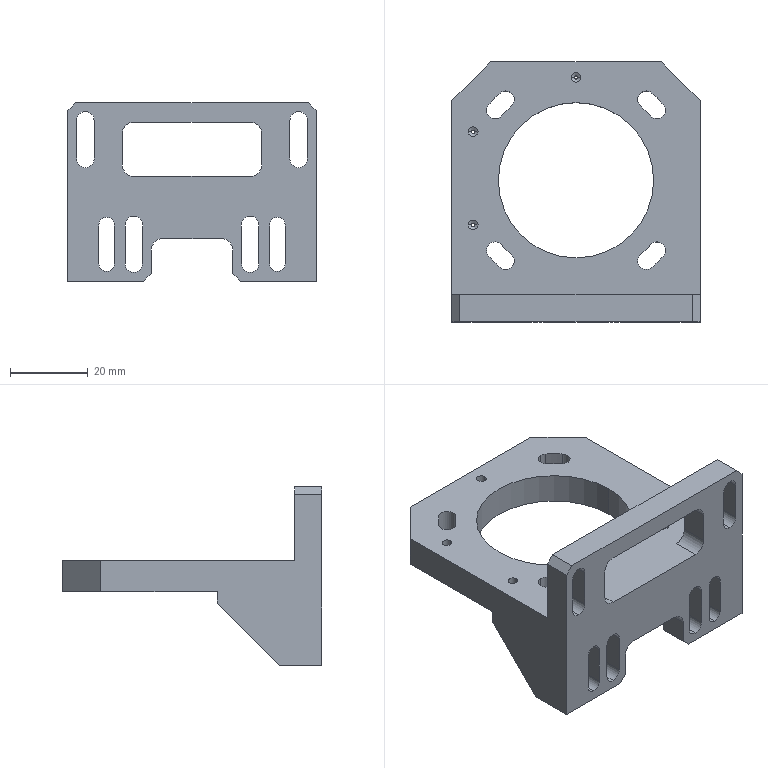NC program | NX | posted with a generic post | part box 64 x 67 x 46 mm
Lines 1 to 508 of 8734:
N10 G17 G21 G94 G90
(ZLEVEL_PROFILE_COPY_3 , TOOL : D10C)
N12 T10 M6
N14 G54
N16 G17 G0 G90 X12.9 Y-10.028 B0. C0. S2500 M3
N18 G43 Z30. H10
N20 Z1.5
N22 G94 G1 Y-9.141 Z1.454 F1000.
N24 X12.902 Y-9.1 Z1.451
N26 X-12.9 Z0.099
N28 Y-12.9 Z-0.1
N30 X12.902 F2500.
N32 X12.9 Y-12.855
N34 Y-9.141
N36 X12.902 Y-9.1
N38 X-12.9
N40 Y-12.9
N42 X-7.171 Z-0.2
N44 X12.902
N46 X12.9 Y-12.855
N48 Y-9.141
N50 X12.902 Y-9.1
N52 X-12.9
N54 Y-12.9
N56 X-7.171 Z-0.3
N58 X12.902
N60 X12.9 Y-12.855
N62 Y-9.141
N64 X12.902 Y-9.1
N66 X-12.9
N68 Y-12.9
N70 X-7.171 Z-0.4
N72 X12.902
N74 X12.9 Y-12.855
N76 Y-9.141
N78 X12.902 Y-9.1
N80 X-12.9
N82 Y-12.9
N84 X-7.171 Z-0.5
N86 X12.902
N88 X12.9 Y-12.855
N90 Y-9.141
N92 X12.902 Y-9.1
N94 X-12.9
N96 Y-12.9
N98 X-7.171 Z-0.6
N100 X12.902
N102 X12.9 Y-12.855
N104 Y-9.141
N106 X12.902 Y-9.1
N108 X-12.9
N110 Y-12.9
N112 X-7.171 Z-0.7
N114 X12.902
N116 X12.9 Y-12.855
N118 Y-9.141
N120 X12.902 Y-9.1
N122 X-12.9
N124 Y-12.9
N126 X-7.171 Z-0.8
N128 X12.902
N130 X12.9 Y-12.855
N132 Y-9.141
N134 X12.902 Y-9.1
N136 X-12.9
N138 Y-12.9
N140 X-7.171 Z-0.9
N142 X12.902
N144 X12.9 Y-12.855
N146 Y-9.141
N148 X12.902 Y-9.1
N150 X-12.9
N152 Y-12.9
N154 X-7.171 Z-1.
N156 X12.902
N158 X12.9 Y-12.855
N160 Y-9.141
N162 X12.902 Y-9.1
N164 X-12.9
N166 Y-12.9
N168 X-7.171 Z-1.1
N170 X12.902
N172 X12.9 Y-12.855
N174 Y-9.141
N176 X12.902 Y-9.1
N178 X-12.9
N180 Y-12.9
N182 X-7.171 Z-1.2
N184 X12.902
N186 X12.9 Y-12.855
N188 Y-9.141
N190 X12.902 Y-9.1
N192 X-12.9
N194 Y-12.9
N196 X-7.171 Z-1.3
N198 X12.902
N200 X12.9 Y-12.855
N202 Y-9.141
N204 X12.902 Y-9.1
N206 X-12.9
N208 Y-12.9
N210 X-7.171 Z-1.4
N212 X12.902
N214 X12.9 Y-12.855
N216 Y-9.141
N218 X12.902 Y-9.1
N220 X-12.9
N222 Y-12.9
N224 X-7.171 Z-1.5
N226 X12.902
N228 X12.9 Y-12.855
N230 Y-9.141
N232 X12.902 Y-9.1
N234 X-12.9
N236 Y-12.9
N238 X-7.171 Z-1.6
N240 X12.902
N242 X12.9 Y-12.855
N244 Y-9.141
N246 X12.902 Y-9.1
N248 X-12.9
N250 Y-12.9
N252 X-7.171 Z-1.7
N254 X12.902
N256 X12.9 Y-12.855
N258 Y-9.141
N260 X12.902 Y-9.1
N262 X-12.9
N264 Y-12.9
N266 X-7.171 Z-1.8
N268 X12.902
N270 X12.9 Y-12.855
N272 Y-9.141
N274 X12.902 Y-9.1
N276 X-12.9
N278 Y-12.9
N280 X-7.171 Z-1.9
N282 X12.902
N284 X12.9 Y-12.855
N286 Y-9.141
N288 X12.902 Y-9.1
N290 X-12.9
N292 Y-12.9
N294 X-7.171 Z-2.
N296 X12.902
N298 X12.9 Y-12.855
N300 Y-9.141
N302 X12.902 Y-9.1
N304 X-12.9
N306 Y-12.9
N308 X-7.171 Z-2.1
N310 X12.902
N312 X12.9 Y-12.855
N314 Y-9.141
N316 X12.902 Y-9.1
N318 X-12.9
N320 Y-12.9
N322 X-7.171 Z-2.2
N324 X12.902
N326 X12.9 Y-12.855
N328 Y-9.141
N330 X12.902 Y-9.1
N332 X-12.9
N334 Y-12.9
N336 X-7.171 Z-2.3
N338 X12.902
N340 X12.9 Y-12.855
N342 Y-9.141
N344 X12.902 Y-9.1
N346 X-12.9
N348 Y-12.9
N350 X-7.171 Z-2.4
N352 X12.902
N354 X12.9 Y-12.855
N356 Y-9.141
N358 X12.902 Y-9.1
N360 X-12.9
N362 Y-12.9
N364 X-7.171 Z-2.5
N366 X12.902
N368 X12.9 Y-12.855
N370 Y-9.141
N372 X12.902 Y-9.1
N374 X-12.9
N376 Y-12.9
N378 X-7.171 Z-2.6
N380 X12.902
N382 X12.9 Y-12.855
N384 Y-9.141
N386 X12.902 Y-9.1
N388 X-12.9
N390 Y-12.9
N392 X-7.171 Z-2.7
N394 X12.902
N396 X12.9 Y-12.855
N398 Y-9.141
N400 X12.902 Y-9.1
N402 X-12.9
N404 Y-12.9
N406 X-7.171 Z-2.8
N408 X12.902
N410 X12.9 Y-12.855
N412 Y-9.141
N414 X12.902 Y-9.1
N416 X-12.9
N418 Y-12.9
N420 X-7.171 Z-2.9
N422 X12.902
N424 X12.9 Y-12.855
N426 Y-9.141
N428 X12.902 Y-9.1
N430 X-12.9
N432 Y-12.9
N434 X-7.171 Z-3.
N436 X12.902
N438 X12.9 Y-12.855
N440 Y-9.141
N442 X12.902 Y-9.1
N444 X-12.9
N446 Y-12.9
N448 X-7.171 Z-3.1
N450 X12.902
N452 X12.9 Y-12.855
N454 Y-9.141
N456 X12.902 Y-9.1
N458 X-12.9
N460 Y-12.9
N462 X-7.171 Z-3.2
N464 X12.902
N466 X12.9 Y-12.855
N468 Y-9.141
N470 X12.902 Y-9.1
N472 X-12.9
N474 Y-12.9
N476 X-7.171 Z-3.3
N478 X12.902
N480 X12.9 Y-12.855
N482 Y-9.141
N484 X12.902 Y-9.1
N486 X-12.9
N488 Y-12.9
N490 X-7.171 Z-3.4
N492 X12.902
N494 X12.9 Y-12.855
N496 Y-9.141
N498 X12.902 Y-9.1
N500 X-12.9
N502 Y-12.9
N504 X-7.171 Z-3.5
N506 X12.902
N508 X12.9 Y-12.855
N510 Y-9.141
N512 X12.902 Y-9.1
N514 X-12.9
N516 Y-12.9
N518 X-7.171 Z-3.6
N520 X12.902
N522 X12.9 Y-12.855
N524 Y-9.141
N526 X12.902 Y-9.1
N528 X-12.9
N530 Y-12.9
N532 X-7.171 Z-3.7
N534 X12.902
N536 X12.9 Y-12.855
N538 Y-9.141
N540 X12.902 Y-9.1
N542 X-12.9
N544 Y-12.9
N546 X-7.171 Z-3.8
N548 X12.902
N550 X12.9 Y-12.855
N552 Y-9.141
N554 X12.902 Y-9.1
N556 X-12.9
N558 Y-12.9
N560 X-7.171 Z-3.9
N562 X12.902
N564 X12.9 Y-12.855
N566 Y-9.141
N568 X12.902 Y-9.1
N570 X-12.9
N572 Y-12.9
N574 X-7.171 Z-4.
N576 X12.902
N578 X12.9 Y-12.855
N580 Y-9.141
N582 X12.902 Y-9.1
N584 X-12.9
N586 Y-12.9
N588 X-7.171 Z-4.1
N590 X12.902
N592 X12.9 Y-12.855
N594 Y-9.141
N596 X12.902 Y-9.1
N598 X-12.9
N600 Y-12.9
N602 X-7.171 Z-4.2
N604 X12.902
N606 X12.9 Y-12.855
N608 Y-9.141
N610 X12.902 Y-9.1
N612 X-12.9
N614 Y-12.9
N616 X-7.171 Z-4.3
N618 X12.902
N620 X12.9 Y-12.855
N622 Y-9.141
N624 X12.902 Y-9.1
N626 X-12.9
N628 Y-12.9
N630 X-7.171 Z-4.4
N632 X12.902
N634 X12.9 Y-12.855
N636 Y-9.141
N638 X12.902 Y-9.1
N640 X-12.9
N642 Y-12.9
N644 X-7.171 Z-4.5
N646 X12.902
N648 X12.9 Y-12.855
N650 Y-9.141
N652 X12.902 Y-9.1
N654 X-12.9
N656 Y-12.9
N658 X-7.171 Z-4.6
N660 X12.902
N662 X12.9 Y-12.855
N664 Y-9.141
N666 X12.902 Y-9.1
N668 X-12.9
N670 Y-12.9
N672 X-7.171 Z-4.7
N674 X12.902
N676 X12.9 Y-12.855
N678 Y-9.141
N680 X12.902 Y-9.1
N682 X-12.9
N684 Y-12.9
N686 X-7.171 Z-4.8
N688 X12.902
N690 X12.9 Y-12.855
N692 Y-9.141
N694 X12.902 Y-9.1
N696 X-12.9
N698 Y-12.9
N700 X-7.171 Z-4.9
N702 X12.902
N704 X12.9 Y-12.855
N706 Y-9.141
N708 X12.902 Y-9.1
N710 X-12.9
N712 Y-12.9
N714 X-7.171 Z-5.
N716 X12.902
N718 X12.9 Y-12.855
N720 Y-9.141
N722 X12.902 Y-9.1
N724 X-12.9
N726 Y-12.9
N728 X-7.171 Z-5.1
N730 X12.902
N732 X12.9 Y-12.855
N734 Y-9.141
N736 X12.902 Y-9.1
N738 X-12.9
N740 Y-12.9
N742 X-7.171 Z-5.2
N744 X12.902
N746 X12.9 Y-12.855
N748 Y-9.141
N750 X12.902 Y-9.1
N752 X-12.9
N754 Y-12.9
N756 X-7.171 Z-5.3
N758 X12.902
N760 X12.9 Y-12.855
N762 Y-9.141
N764 X12.902 Y-9.1
N766 X-12.9
N768 Y-12.9
N770 X-7.171 Z-5.4
N772 X12.902
N774 X12.9 Y-12.855
N776 Y-9.141
N778 X12.902 Y-9.1
N780 X-12.9
N782 Y-12.9
N784 X-7.171 Z-5.5
N786 X12.902
N788 X12.9 Y-12.855
N790 Y-9.141
N792 X12.902 Y-9.1
N794 X-12.9
N796 Y-12.9
N798 X-7.171 Z-5.6
N800 X12.902
N802 X12.9 Y-12.855
N804 Y-9.141
N806 X12.902 Y-9.1
N808 X-12.9
N810 Y-12.9
N812 X-7.171 Z-5.7
N814 X12.902
N816 X12.9 Y-12.855
N818 Y-9.141
N820 X12.902 Y-9.1
N822 X-12.9
N824 Y-12.9
N826 X-7.171 Z-5.8
N828 X12.902
N830 X12.9 Y-12.855
N832 Y-9.141
N834 X12.902 Y-9.1
N836 X-12.9
N838 Y-12.9
N840 X-7.171 Z-5.9
N842 X12.902
N844 X12.9 Y-12.855
N846 Y-9.141
N848 X12.902 Y-9.1
N850 X-12.9
N852 Y-12.9
N854 X-7.171 Z-6.
N856 X12.902
N858 X12.9 Y-12.855
N860 Y-9.141
N862 X12.902 Y-9.1
N864 X-12.9
N866 Y-12.9
N868 X-7.171 Z-6.1
N870 X12.902
N872 X12.9 Y-12.855
N874 Y-9.141
N876 X12.902 Y-9.1
N878 X-12.9
N880 Y-12.9
N882 X-7.171 Z-6.2
N884 X12.902
N886 X12.9 Y-12.855
N888 Y-9.141
N890 X12.902 Y-9.1
N892 X-12.9
N894 Y-12.9
N896 X-7.171 Z-6.3
N898 X12.902
N900 X12.9 Y-12.855
N902 Y-9.141
N904 X12.902 Y-9.1
N906 X-12.9
N908 Y-12.9
N910 X-7.171 Z-6.4
N912 X12.902
N914 X12.9 Y-12.855
N916 Y-9.141
N918 X12.902 Y-9.1
N920 X-12.9
N922 Y-12.9
N924 X-7.171 Z-6.5
N926 X12.902
N928 X12.9 Y-12.855
N930 Y-9.141
N932 X12.902 Y-9.1
N934 X-12.9
N936 Y-12.9
N938 X-7.171 Z-6.6
N940 X12.902
N942 X12.9 Y-12.855
N944 Y-9.141
N946 X12.902 Y-9.1
N948 X-12.9
N950 Y-12.9
N952 X-7.171 Z-6.7
N954 X12.902
N956 X12.9 Y-12.855
N958 Y-9.141
N960 X12.902 Y-9.1
N962 X-12.9
N964 Y-12.9
N966 X-7.171 Z-6.8
N968 X12.902
N970 X12.9 Y-12.855
N972 Y-9.141
N974 X12.902 Y-9.1
N976 X-12.9
N978 Y-12.9
N980 X-7.171 Z-6.9
N982 X12.902
N984 X12.9 Y-12.855
N986 Y-9.141
N988 X12.902 Y-9.1
N990 X-12.9
N992 Y-12.9
N994 X-7.171 Z-7.
N996 X12.902
N998 X12.9 Y-12.855
N1000 Y-9.141
N1002 X12.902 Y-9.1
N1004 X-12.9
N1006 Y-12.9
N1008 X-7.171
N1010 Z-5.5
N1012 G0 Z30.
N1014 M5